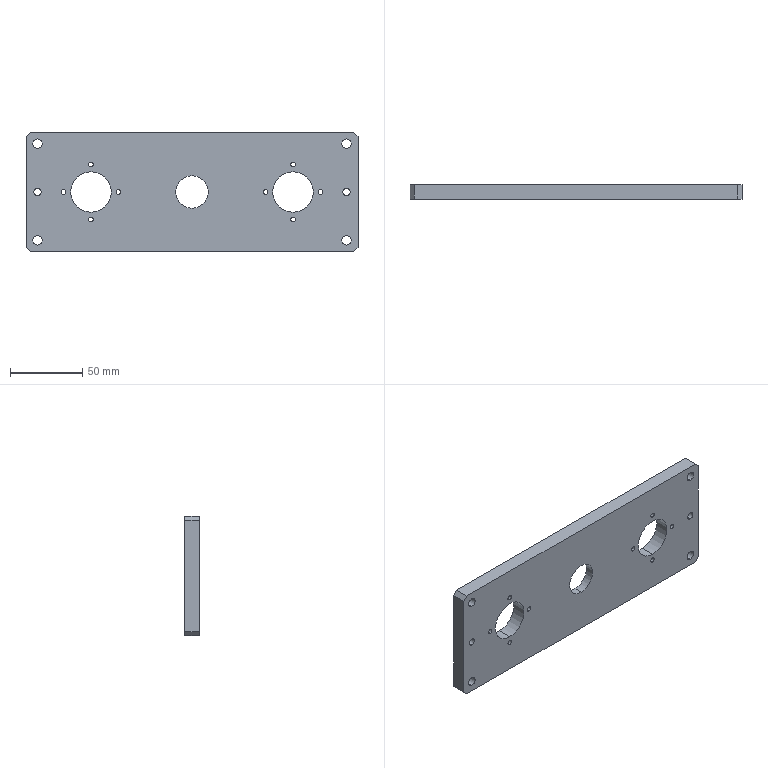Part | STEP file | PN_0016 | 1 solid | 53 faces | box 230 x 10 x 83 mm | volume 156846 mm3 | cylinder 38 | plane 15 | commonest cylinder face diameters 3.3 x16 6.5 x8 5 x4 6 x4 28 x4 22.5 x2